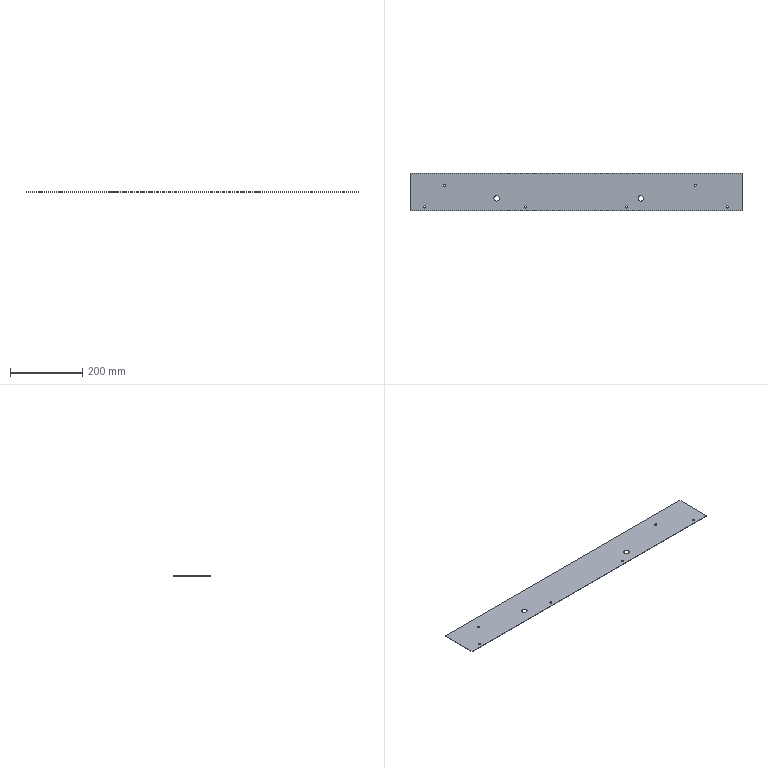Part | SolidWorks | features Cut 1, Extrusion 1, HoleWzd 1 | 1 solid | 22 faces | box 920 x 105 x 1 mm | volume 96077 mm3 | cylinder 16 | plane 6 | commonest cylinder face diameters 6 x12 15 x4
STEP:
#1=CARTESIAN_POINT('',(-423.,-41.5,-0.5));
#2=VERTEX_POINT('',#1);
#3=CARTESIAN_POINT('',(-417.,-41.5,-0.5));
#4=VERTEX_POINT('',#3);
#5=CARTESIAN_POINT('',(-420.,-41.5,-0.5));
#6=DIRECTION('',(0.,0.,1.));
#7=DIRECTION('',(1.,0.,0.));
#8=AXIS2_PLACEMENT_3D('',#5,#6,#7);
#9=CIRCLE('',#8,3.);
#10=EDGE_CURVE('',#2,#4,#9,.T.);
#11=ORIENTED_EDGE('',*,*,#10,.F.);
#12=CARTESIAN_POINT('',(-423.,-41.5,0.5));
#13=VERTEX_POINT('',#12);
#14=CARTESIAN_POINT('',(-423.,-41.5,0.5));
#15=DIRECTION('',(0.,0.,1.));
#16=VECTOR('',#15,1000.);
#17=LINE('',#14,#16);
#18=EDGE_CURVE('',#2,#13,#17,.T.);
#19=ORIENTED_EDGE('',*,*,#18,.T.);
#20=CARTESIAN_POINT('',(-417.,-41.5,0.5));
#21=VERTEX_POINT('',#20);
#22=CARTESIAN_POINT('',(-420.,-41.5,0.5));
#23=DIRECTION('',(0.,0.,1.));
#24=DIRECTION('',(1.,0.,0.));
#25=AXIS2_PLACEMENT_3D('',#22,#23,#24);
#26=CIRCLE('',#25,3.);
#27=EDGE_CURVE('',#13,#21,#26,.T.);
#28=ORIENTED_EDGE('',*,*,#27,.T.);
#29=CARTESIAN_POINT('',(-417.,-41.5,0.5));
#30=DIRECTION('',(0.,0.,1.));
#31=VECTOR('',#30,1000.);
#32=LINE('',#29,#31);
#33=EDGE_CURVE('',#4,#21,#32,.T.);
#34=ORIENTED_EDGE('',*,*,#33,.F.);
#35=EDGE_LOOP('',(#11,#19,#28,#34));
#36=FACE_OUTER_BOUND('',#35,.T.);
#37=CARTESIAN_POINT('',(-420.,-41.5,0.5));
#38=DIRECTION('',(0.,0.,1.));
#39=DIRECTION('',(1.,0.,0.));
#40=AXIS2_PLACEMENT_3D('',#37,#38,#39);
#41=CYLINDRICAL_SURFACE('',#40,3.);
#42=ADVANCED_FACE('',(#36),#41,.F.);
#43=CARTESIAN_POINT('',(-143.,-41.5,-0.5));
#44=VERTEX_POINT('',#43);
#45=CARTESIAN_POINT('',(-137.,-41.5,-0.5));
#46=VERTEX_POINT('',#45);
#47=CARTESIAN_POINT('',(-140.,-41.5,-0.5));
#48=DIRECTION('',(0.,0.,1.));
#49=DIRECTION('',(1.,0.,0.));
#50=AXIS2_PLACEMENT_3D('',#47,#48,#49);
#51=CIRCLE('',#50,3.);
#52=EDGE_CURVE('',#44,#46,#51,.T.);
#53=ORIENTED_EDGE('',*,*,#52,.F.);
#54=CARTESIAN_POINT('',(-143.,-41.5,0.5));
#55=VERTEX_POINT('',#54);
#56=CARTESIAN_POINT('',(-143.,-41.5,0.5));
#57=DIRECTION('',(0.,0.,1.));
#58=VECTOR('',#57,1000.);
#59=LINE('',#56,#58);
#60=EDGE_CURVE('',#44,#55,#59,.T.);
#61=ORIENTED_EDGE('',*,*,#60,.T.);
#62=CARTESIAN_POINT('',(-137.,-41.5,0.5));
#63=VERTEX_POINT('',#62);
#64=CARTESIAN_POINT('',(-140.,-41.5,0.5));
#65=DIRECTION('',(0.,0.,1.));
#66=DIRECTION('',(1.,0.,0.));
#67=AXIS2_PLACEMENT_3D('',#64,#65,#66);
#68=CIRCLE('',#67,3.);
#69=EDGE_CURVE('',#55,#63,#68,.T.);
#70=ORIENTED_EDGE('',*,*,#69,.T.);
#71=CARTESIAN_POINT('',(-137.,-41.5,0.5));
#72=DIRECTION('',(0.,0.,1.));
#73=VECTOR('',#72,1000.);
#74=LINE('',#71,#73);
#75=EDGE_CURVE('',#46,#63,#74,.T.);
#76=ORIENTED_EDGE('',*,*,#75,.F.);
#77=EDGE_LOOP('',(#53,#61,#70,#76));
#78=FACE_OUTER_BOUND('',#77,.T.);
#79=CARTESIAN_POINT('',(-140.,-41.5,0.5));
#80=DIRECTION('',(0.,0.,1.));
#81=DIRECTION('',(1.,0.,0.));
#82=AXIS2_PLACEMENT_3D('',#79,#80,#81);
#83=CYLINDRICAL_SURFACE('',#82,3.);
#84=ADVANCED_FACE('',(#78),#83,.F.);
#85=CARTESIAN_POINT('',(137.,-41.5,-0.5));
#86=VERTEX_POINT('',#85);
#87=CARTESIAN_POINT('',(143.,-41.5,-0.5));
#88=VERTEX_POINT('',#87);
#89=CARTESIAN_POINT('',(140.,-41.5,-0.5));
#90=DIRECTION('',(0.,0.,1.));
#91=DIRECTION('',(1.,0.,0.));
#92=AXIS2_PLACEMENT_3D('',#89,#90,#91);
#93=CIRCLE('',#92,3.);
#94=EDGE_CURVE('',#86,#88,#93,.T.);
#95=ORIENTED_EDGE('',*,*,#94,.F.);
#96=CARTESIAN_POINT('',(137.,-41.5,0.5));
#97=VERTEX_POINT('',#96);
#98=CARTESIAN_POINT('',(137.,-41.5,0.5));
#99=DIRECTION('',(0.,0.,1.));
#100=VECTOR('',#99,1000.);
#101=LINE('',#98,#100);
#102=EDGE_CURVE('',#86,#97,#101,.T.);
#103=ORIENTED_EDGE('',*,*,#102,.T.);
#104=CARTESIAN_POINT('',(143.,-41.5,0.5));
#105=VERTEX_POINT('',#104);
#106=CARTESIAN_POINT('',(140.,-41.5,0.5));
#107=DIRECTION('',(0.,0.,1.));
#108=DIRECTION('',(1.,0.,0.));
#109=AXIS2_PLACEMENT_3D('',#106,#107,#108);
#110=CIRCLE('',#109,3.);
#111=EDGE_CURVE('',#97,#105,#110,.T.);
#112=ORIENTED_EDGE('',*,*,#111,.T.);
#113=CARTESIAN_POINT('',(143.,-41.5,0.5));
#114=DIRECTION('',(0.,0.,1.));
#115=VECTOR('',#114,1000.);
#116=LINE('',#113,#115);
#117=EDGE_CURVE('',#88,#105,#116,.T.);
#118=ORIENTED_EDGE('',*,*,#117,.F.);
#119=EDGE_LOOP('',(#95,#103,#112,#118));
#120=FACE_OUTER_BOUND('',#119,.T.);
#121=CARTESIAN_POINT('',(140.,-41.5,0.5));
#122=DIRECTION('',(0.,0.,1.));
#123=DIRECTION('',(1.,0.,0.));
#124=AXIS2_PLACEMENT_3D('',#121,#122,#123);
#125=CYLINDRICAL_SURFACE('',#124,3.);
#126=ADVANCED_FACE('',(#120),#125,.F.);
#127=CARTESIAN_POINT('',(-368.,18.5,-0.5));
#128=VERTEX_POINT('',#127);
#129=CARTESIAN_POINT('',(-362.,18.5,-0.5));
#130=VERTEX_POINT('',#129);
#131=CARTESIAN_POINT('',(-365.,18.5,-0.5));
#132=DIRECTION('',(0.,0.,1.));
#133=DIRECTION('',(1.,0.,0.));
#134=AXIS2_PLACEMENT_3D('',#131,#132,#133);
#135=CIRCLE('',#134,3.);
#136=EDGE_CURVE('',#128,#130,#135,.T.);
#137=ORIENTED_EDGE('',*,*,#136,.F.);
#138=CARTESIAN_POINT('',(-368.,18.5,0.5));
#139=VERTEX_POINT('',#138);
#140=CARTESIAN_POINT('',(-368.,18.5,0.5));
#141=DIRECTION('',(0.,0.,1.));
#142=VECTOR('',#141,1000.);
#143=LINE('',#140,#142);
#144=EDGE_CURVE('',#128,#139,#143,.T.);
#145=ORIENTED_EDGE('',*,*,#144,.T.);
#146=CARTESIAN_POINT('',(-362.,18.5,0.5));
#147=VERTEX_POINT('',#146);
#148=CARTESIAN_POINT('',(-365.,18.5,0.5));
#149=DIRECTION('',(0.,0.,1.));
#150=DIRECTION('',(1.,0.,0.));
#151=AXIS2_PLACEMENT_3D('',#148,#149,#150);
#152=CIRCLE('',#151,3.);
#153=EDGE_CURVE('',#139,#147,#152,.T.);
#154=ORIENTED_EDGE('',*,*,#153,.T.);
#155=CARTESIAN_POINT('',(-362.,18.5,0.5));
#156=DIRECTION('',(0.,0.,1.));
#157=VECTOR('',#156,1000.);
#158=LINE('',#155,#157);
#159=EDGE_CURVE('',#130,#147,#158,.T.);
#160=ORIENTED_EDGE('',*,*,#159,.F.);
#161=EDGE_LOOP('',(#137,#145,#154,#160));
#162=FACE_OUTER_BOUND('',#161,.T.);
#163=CARTESIAN_POINT('',(-365.,18.5,0.5));
#164=DIRECTION('',(0.,0.,1.));
#165=DIRECTION('',(1.,0.,0.));
#166=AXIS2_PLACEMENT_3D('',#163,#164,#165);
#167=CYLINDRICAL_SURFACE('',#166,3.);
#168=ADVANCED_FACE('',(#162),#167,.F.);
#169=CARTESIAN_POINT('',(327.,18.5,-0.5));
#170=VERTEX_POINT('',#169);
#171=CARTESIAN_POINT('',(333.,18.5,-0.5));
#172=VERTEX_POINT('',#171);
#173=CARTESIAN_POINT('',(330.,18.5,-0.5));
#174=DIRECTION('',(0.,0.,1.));
#175=DIRECTION('',(1.,0.,0.));
#176=AXIS2_PLACEMENT_3D('',#173,#174,#175);
#177=CIRCLE('',#176,3.);
#178=EDGE_CURVE('',#170,#172,#177,.T.);
#179=ORIENTED_EDGE('',*,*,#178,.F.);
#180=CARTESIAN_POINT('',(327.,18.5,0.5));
#181=VERTEX_POINT('',#180);
#182=CARTESIAN_POINT('',(327.,18.5,0.5));
#183=DIRECTION('',(0.,0.,1.));
#184=VECTOR('',#183,1000.);
#185=LINE('',#182,#184);
#186=EDGE_CURVE('',#170,#181,#185,.T.);
#187=ORIENTED_EDGE('',*,*,#186,.T.);
#188=CARTESIAN_POINT('',(333.,18.5,0.5));
#189=VERTEX_POINT('',#188);
#190=CARTESIAN_POINT('',(330.,18.5,0.5));
#191=DIRECTION('',(0.,0.,1.));
#192=DIRECTION('',(1.,0.,0.));
#193=AXIS2_PLACEMENT_3D('',#190,#191,#192);
#194=CIRCLE('',#193,3.);
#195=EDGE_CURVE('',#181,#189,#194,.T.);
#196=ORIENTED_EDGE('',*,*,#195,.T.);
#197=CARTESIAN_POINT('',(333.,18.5,0.5));
#198=DIRECTION('',(0.,0.,1.));
#199=VECTOR('',#198,1000.);
#200=LINE('',#197,#199);
#201=EDGE_CURVE('',#172,#189,#200,.T.);
#202=ORIENTED_EDGE('',*,*,#201,.F.);
#203=EDGE_LOOP('',(#179,#187,#196,#202));
#204=FACE_OUTER_BOUND('',#203,.T.);
#205=CARTESIAN_POINT('',(330.,18.5,0.5));
#206=DIRECTION('',(0.,0.,1.));
#207=DIRECTION('',(1.,0.,0.));
#208=AXIS2_PLACEMENT_3D('',#205,#206,#207);
#209=CYLINDRICAL_SURFACE('',#208,3.);
#210=ADVANCED_FACE('',(#204),#209,.F.);
#211=CARTESIAN_POINT('',(417.,-41.5,-0.5));
#212=VERTEX_POINT('',#211);
#213=CARTESIAN_POINT('',(423.,-41.5,-0.5));
#214=VERTEX_POINT('',#213);
#215=CARTESIAN_POINT('',(420.,-41.5,-0.5));
#216=DIRECTION('',(0.,0.,1.));
#217=DIRECTION('',(1.,0.,0.));
#218=AXIS2_PLACEMENT_3D('',#215,#216,#217);
#219=CIRCLE('',#218,3.);
#220=EDGE_CURVE('',#212,#214,#219,.T.);
#221=ORIENTED_EDGE('',*,*,#220,.F.);
#222=CARTESIAN_POINT('',(417.,-41.5,0.5));
#223=VERTEX_POINT('',#222);
#224=CARTESIAN_POINT('',(417.,-41.5,0.5));
#225=DIRECTION('',(0.,0.,1.));
#226=VECTOR('',#225,1000.);
#227=LINE('',#224,#226);
#228=EDGE_CURVE('',#212,#223,#227,.T.);
#229=ORIENTED_EDGE('',*,*,#228,.T.);
#230=CARTESIAN_POINT('',(423.,-41.5,0.5));
#231=VERTEX_POINT('',#230);
#232=CARTESIAN_POINT('',(420.,-41.5,0.5));
#233=DIRECTION('',(0.,0.,1.));
#234=DIRECTION('',(1.,0.,0.));
#235=AXIS2_PLACEMENT_3D('',#232,#233,#234);
#236=CIRCLE('',#235,3.);
#237=EDGE_CURVE('',#223,#231,#236,.T.);
#238=ORIENTED_EDGE('',*,*,#237,.T.);
#239=CARTESIAN_POINT('',(423.,-41.5,0.5));
#240=DIRECTION('',(0.,0.,1.));
#241=VECTOR('',#240,1000.);
#242=LINE('',#239,#241);
#243=EDGE_CURVE('',#214,#231,#242,.T.);
#244=ORIENTED_EDGE('',*,*,#243,.F.);
#245=EDGE_LOOP('',(#221,#229,#238,#244));
#246=FACE_OUTER_BOUND('',#245,.T.);
#247=CARTESIAN_POINT('',(420.,-41.5,0.5));
#248=DIRECTION('',(0.,0.,1.));
#249=DIRECTION('',(1.,0.,0.));
#250=AXIS2_PLACEMENT_3D('',#247,#248,#249);
#251=CYLINDRICAL_SURFACE('',#250,3.);
#252=ADVANCED_FACE('',(#246),#251,.F.);
#253=CARTESIAN_POINT('',(172.5,-17.5,-0.5));
#254=VERTEX_POINT('',#253);
#255=CARTESIAN_POINT('',(187.5,-17.5,-0.5));
#256=VERTEX_POINT('',#255);
#257=CARTESIAN_POINT('',(180.,-17.5,-0.5));
#258=DIRECTION('',(0.,0.,1.));
#259=DIRECTION('',(1.,0.,0.));
#260=AXIS2_PLACEMENT_3D('',#257,#258,#259);
#261=CIRCLE('',#260,7.5);
#262=EDGE_CURVE('',#254,#256,#261,.T.);
#263=ORIENTED_EDGE('',*,*,#262,.F.);
#264=CARTESIAN_POINT('',(172.5,-17.5,0.5));
#265=VERTEX_POINT('',#264);
#266=CARTESIAN_POINT('',(172.5,-17.5,-0.5));
#267=DIRECTION('',(0.,0.,1.));
#268=VECTOR('',#267,1000.);
#269=LINE('',#266,#268);
#270=EDGE_CURVE('',#254,#265,#269,.T.);
#271=ORIENTED_EDGE('',*,*,#270,.T.);
#272=CARTESIAN_POINT('',(187.5,-17.5,0.5));
#273=VERTEX_POINT('',#272);
#274=CARTESIAN_POINT('',(180.,-17.5,0.5));
#275=DIRECTION('',(0.,0.,1.));
#276=DIRECTION('',(1.,0.,0.));
#277=AXIS2_PLACEMENT_3D('',#274,#275,#276);
#278=CIRCLE('',#277,7.5);
#279=EDGE_CURVE('',#265,#273,#278,.T.);
#280=ORIENTED_EDGE('',*,*,#279,.T.);
#281=CARTESIAN_POINT('',(187.5,-17.5,-0.5));
#282=DIRECTION('',(0.,0.,1.));
#283=VECTOR('',#282,1000.);
#284=LINE('',#281,#283);
#285=EDGE_CURVE('',#256,#273,#284,.T.);
#286=ORIENTED_EDGE('',*,*,#285,.F.);
#287=EDGE_LOOP('',(#263,#271,#280,#286));
#288=FACE_OUTER_BOUND('',#287,.T.);
#289=CARTESIAN_POINT('',(180.,-17.5,-0.5));
#290=DIRECTION('',(0.,0.,1.));
#291=DIRECTION('',(1.,0.,0.));
#292=AXIS2_PLACEMENT_3D('',#289,#290,#291);
#293=CYLINDRICAL_SURFACE('',#292,7.5);
#294=ADVANCED_FACE('',(#288),#293,.F.);
#295=CARTESIAN_POINT('',(-227.5,-17.5,-0.5));
#296=VERTEX_POINT('',#295);
#297=CARTESIAN_POINT('',(-212.5,-17.5,-0.5));
#298=VERTEX_POINT('',#297);
#299=CARTESIAN_POINT('',(-220.,-17.5,-0.5));
#300=DIRECTION('',(0.,0.,1.));
#301=DIRECTION('',(1.,0.,0.));
#302=AXIS2_PLACEMENT_3D('',#299,#300,#301);
#303=CIRCLE('',#302,7.5);
#304=EDGE_CURVE('',#296,#298,#303,.T.);
#305=ORIENTED_EDGE('',*,*,#304,.F.);
#306=CARTESIAN_POINT('',(-227.5,-17.5,0.5));
#307=VERTEX_POINT('',#306);
#308=CARTESIAN_POINT('',(-227.5,-17.5,-0.5));
#309=DIRECTION('',(0.,0.,1.));
#310=VECTOR('',#309,1000.);
#311=LINE('',#308,#310);
#312=EDGE_CURVE('',#296,#307,#311,.T.);
#313=ORIENTED_EDGE('',*,*,#312,.T.);
#314=CARTESIAN_POINT('',(-212.5,-17.5,0.5));
#315=VERTEX_POINT('',#314);
#316=CARTESIAN_POINT('',(-220.,-17.5,0.5));
#317=DIRECTION('',(0.,0.,1.));
#318=DIRECTION('',(1.,0.,0.));
#319=AXIS2_PLACEMENT_3D('',#316,#317,#318);
#320=CIRCLE('',#319,7.5);
#321=EDGE_CURVE('',#307,#315,#320,.T.);
#322=ORIENTED_EDGE('',*,*,#321,.T.);
#323=CARTESIAN_POINT('',(-212.5,-17.5,-0.5));
#324=DIRECTION('',(0.,0.,1.));
#325=VECTOR('',#324,1000.);
#326=LINE('',#323,#325);
#327=EDGE_CURVE('',#298,#315,#326,.T.);
#328=ORIENTED_EDGE('',*,*,#327,.F.);
#329=EDGE_LOOP('',(#305,#313,#322,#328));
#330=FACE_OUTER_BOUND('',#329,.T.);
#331=CARTESIAN_POINT('',(-220.,-17.5,-0.5));
#332=DIRECTION('',(0.,0.,1.));
#333=DIRECTION('',(1.,0.,0.));
#334=AXIS2_PLACEMENT_3D('',#331,#332,#333);
#335=CYLINDRICAL_SURFACE('',#334,7.5);
#336=ADVANCED_FACE('',(#330),#335,.F.);
#337=CARTESIAN_POINT('',(-460.,-52.5,-0.5));
#338=VERTEX_POINT('',#337);
#339=CARTESIAN_POINT('',(-460.,-52.5,0.5));
#340=VERTEX_POINT('',#339);
#341=CARTESIAN_POINT('',(-460.,-52.5,-0.5));
#342=DIRECTION('',(0.,0.,1.));
#343=VECTOR('',#342,1000.);
#344=LINE('',#341,#343);
#345=EDGE_CURVE('',#338,#340,#344,.T.);
#346=ORIENTED_EDGE('',*,*,#345,.T.);
#347=CARTESIAN_POINT('',(-460.,52.5,0.5));
#348=VERTEX_POINT('',#347);
#349=CARTESIAN_POINT('',(-460.,52.5,0.5));
#350=DIRECTION('',(0.,-1.,0.));
#351=VECTOR('',#350,1000.);
#352=LINE('',#349,#351);
#353=EDGE_CURVE('',#348,#340,#352,.T.);
#354=ORIENTED_EDGE('',*,*,#353,.F.);
#355=CARTESIAN_POINT('',(-460.,52.5,-0.5));
#356=VERTEX_POINT('',#355);
#357=CARTESIAN_POINT('',(-460.,52.5,-0.5));
#358=DIRECTION('',(0.,0.,1.));
#359=VECTOR('',#358,1000.);
#360=LINE('',#357,#359);
#361=EDGE_CURVE('',#356,#348,#360,.T.);
#362=ORIENTED_EDGE('',*,*,#361,.F.);
#363=CARTESIAN_POINT('',(-460.,52.5,-0.5));
#364=DIRECTION('',(0.,-1.,0.));
#365=VECTOR('',#364,1000.);
#366=LINE('',#363,#365);
#367=EDGE_CURVE('',#356,#338,#366,.T.);
#368=ORIENTED_EDGE('',*,*,#367,.T.);
#369=EDGE_LOOP('',(#346,#354,#362,#368));
#370=FACE_OUTER_BOUND('',#369,.T.);
#371=CARTESIAN_POINT('',(-460.,52.5,-0.5));
#372=DIRECTION('',(1.,0.,0.));
#373=DIRECTION('',(0.,0.,-1.));
#374=AXIS2_PLACEMENT_3D('',#371,#372,#373);
#375=PLANE('',#374);
#376=ADVANCED_FACE('',(#370),#375,.F.);
#377=CARTESIAN_POINT('',(-420.,-41.5,0.5));
#378=DIRECTION('',(0.,0.,1.));
#379=DIRECTION('',(1.,0.,0.));
#380=AXIS2_PLACEMENT_3D('',#377,#378,#379);
#381=CIRCLE('',#380,3.);
#382=EDGE_CURVE('',#21,#13,#381,.T.);
#383=ORIENTED_EDGE('',*,*,#382,.F.);
#384=ORIENTED_EDGE('',*,*,#27,.F.);
#385=EDGE_LOOP('',(#383,#384));
#386=FACE_BOUND('',#385,.T.);
#387=CARTESIAN_POINT('',(-140.,-41.5,0.5));
#388=DIRECTION('',(0.,0.,1.));
#389=DIRECTION('',(1.,0.,0.));
#390=AXIS2_PLACEMENT_3D('',#387,#388,#389);
#391=CIRCLE('',#390,3.);
#392=EDGE_CURVE('',#63,#55,#391,.T.);
#393=ORIENTED_EDGE('',*,*,#392,.F.);
#394=ORIENTED_EDGE('',*,*,#69,.F.);
#395=EDGE_LOOP('',(#393,#394));
#396=FACE_BOUND('',#395,.T.);
#397=CARTESIAN_POINT('',(140.,-41.5,0.5));
#398=DIRECTION('',(0.,0.,1.));
#399=DIRECTION('',(1.,0.,0.));
#400=AXIS2_PLACEMENT_3D('',#397,#398,#399);
#401=CIRCLE('',#400,3.);
#402=EDGE_CURVE('',#105,#97,#401,.T.);
#403=ORIENTED_EDGE('',*,*,#402,.F.);
#404=ORIENTED_EDGE('',*,*,#111,.F.);
#405=EDGE_LOOP('',(#403,#404));
#406=FACE_BOUND('',#405,.T.);
#407=CARTESIAN_POINT('',(-365.,18.5,0.5));
#408=DIRECTION('',(0.,0.,1.));
#409=DIRECTION('',(1.,0.,0.));
#410=AXIS2_PLACEMENT_3D('',#407,#408,#409);
#411=CIRCLE('',#410,3.);
#412=EDGE_CURVE('',#147,#139,#411,.T.);
#413=ORIENTED_EDGE('',*,*,#412,.F.);
#414=ORIENTED_EDGE('',*,*,#153,.F.);
#415=EDGE_LOOP('',(#413,#414));
#416=FACE_BOUND('',#415,.T.);
#417=CARTESIAN_POINT('',(330.,18.5,0.5));
#418=DIRECTION('',(0.,0.,1.));
#419=DIRECTION('',(1.,0.,0.));
#420=AXIS2_PLACEMENT_3D('',#417,#418,#419);
#421=CIRCLE('',#420,3.);
#422=EDGE_CURVE('',#189,#181,#421,.T.);
#423=ORIENTED_EDGE('',*,*,#422,.F.);
#424=ORIENTED_EDGE('',*,*,#195,.F.);
#425=EDGE_LOOP('',(#423,#424));
#426=FACE_BOUND('',#425,.T.);
#427=CARTESIAN_POINT('',(420.,-41.5,0.5));
#428=DIRECTION('',(0.,0.,1.));
#429=DIRECTION('',(1.,0.,0.));
#430=AXIS2_PLACEMENT_3D('',#427,#428,#429);
#431=CIRCLE('',#430,3.);
#432=EDGE_CURVE('',#231,#223,#431,.T.);
#433=ORIENTED_EDGE('',*,*,#432,.F.);
#434=ORIENTED_EDGE('',*,*,#237,.F.);
#435=EDGE_LOOP('',(#433,#434));
#436=FACE_BOUND('',#435,.T.);
#437=CARTESIAN_POINT('',(180.,-17.5,0.5));
#438=DIRECTION('',(0.,0.,1.));
#439=DIRECTION('',(1.,0.,0.));
#440=AXIS2_PLACEMENT_3D('',#437,#438,#439);
#441=CIRCLE('',#440,7.5);
#442=EDGE_CURVE('',#273,#265,#441,.T.);
#443=ORIENTED_EDGE('',*,*,#442,.F.);
#444=ORIENTED_EDGE('',*,*,#279,.F.);
#445=EDGE_LOOP('',(#443,#444));
#446=FACE_BOUND('',#445,.T.);
#447=CARTESIAN_POINT('',(-220.,-17.5,0.5));
#448=DIRECTION('',(0.,0.,1.));
#449=DIRECTION('',(1.,0.,0.));
#450=AXIS2_PLACEMENT_3D('',#447,#448,#449);
#451=CIRCLE('',#450,7.5);
#452=EDGE_CURVE('',#315,#307,#451,.T.);
#453=ORIENTED_EDGE('',*,*,#452,.F.);
#454=ORIENTED_EDGE('',*,*,#321,.F.);
#455=EDGE_LOOP('',(#453,#454));
#456=FACE_BOUND('',#455,.T.);
#457=CARTESIAN_POINT('',(460.,-52.5,0.5));
#458=VERTEX_POINT('',#457);
#459=CARTESIAN_POINT('',(-460.,-52.5,0.5));
#460=DIRECTION('',(1.,0.,0.));
#461=VECTOR('',#460,1000.);
#462=LINE('',#459,#461);
#463=EDGE_CURVE('',#340,#458,#462,.T.);
#464=ORIENTED_EDGE('',*,*,#463,.T.);
#465=CARTESIAN_POINT('',(460.,52.5,0.5));
#466=VERTEX_POINT('',#465);
#467=CARTESIAN_POINT('',(460.,52.5,0.5));
#468=DIRECTION('',(0.,-1.,0.));
#469=VECTOR('',#468,1000.);
#470=LINE('',#467,#469);
#471=EDGE_CURVE('',#466,#458,#470,.T.);
#472=ORIENTED_EDGE('',*,*,#471,.F.);
#473=CARTESIAN_POINT('',(-460.,52.5,0.5));
#474=DIRECTION('',(1.,0.,0.));
#475=VECTOR('',#474,1000.);
#476=LINE('',#473,#475);
#477=EDGE_CURVE('',#348,#466,#476,.T.);
#478=ORIENTED_EDGE('',*,*,#477,.F.);
#479=ORIENTED_EDGE('',*,*,#353,.T.);
#480=EDGE_LOOP('',(#464,#472,#478,#479));
#481=FACE_OUTER_BOUND('',#480,.T.);
#482=CARTESIAN_POINT('',(-460.,52.5,0.5));
#483=DIRECTION('',(0.,0.,-1.));
#484=DIRECTION('',(-1.,0.,0.));
#485=AXIS2_PLACEMENT_3D('',#482,#483,#484);
#486=PLANE('',#485);
#487=ADVANCED_FACE('',(#386,#396,#406,#416,#426,#436,#446,#456,#481),#486,.F.);
#488=CARTESIAN_POINT('',(460.,-52.5,-0.5));
#489=VERTEX_POINT('',#488);
#490=CARTESIAN_POINT('',(460.,-52.5,-0.5));
#491=DIRECTION('',(0.,0.,-1.));
#492=VECTOR('',#491,1000.);
#493=LINE('',#490,#492);
#494=EDGE_CURVE('',#458,#489,#493,.T.);
#495=ORIENTED_EDGE('',*,*,#494,.T.);
#496=CARTESIAN_POINT('',(460.,52.5,-0.5));
#497=VERTEX_POINT('',#496);
#498=CARTESIAN_POINT('',(460.,52.5,-0.5));
#499=DIRECTION('',(0.,-1.,0.));
#500=VECTOR('',#499,1000.);
#501=LINE('',#498,#500);
#502=EDGE_CURVE('',#497,#489,#501,.T.);
#503=ORIENTED_EDGE('',*,*,#502,.F.);
#504=CARTESIAN_POINT('',(460.,52.5,-0.5));
#505=DIRECTION('',(0.,0.,-1.));
#506=VECTOR('',#505,1000.);
#507=LINE('',#504,#506);
#508=EDGE_CURVE('',#466,#497,#507,.T.);
#509=ORIENTED_EDGE('',*,*,#508,.F.);
#510=ORIENTED_EDGE('',*,*,#471,.T.);
#511=EDGE_LOOP('',(#495,#503,#509,#510));
#512=FACE_OUTER_BOUND('',#511,.T.);
#513=CARTESIAN_POINT('',(460.,52.5,-0.5));
#514=DIRECTION('',(-1.,0.,0.));
#515=DIRECTION('',(0.,0.,1.));
#516=AXIS2_PLACEMENT_3D('',#513,#514,#515);
#517=PLANE('',#516);
#518=ADVANCED_FACE('',(#512),#517,.F.);
#519=CARTESIAN_POINT('',(-420.,-41.5,-0.5));
#520=DIRECTION('',(0.,0.,1.));
#521=DIRECTION('',(1.,0.,0.));
#522=AXIS2_PLACEMENT_3D('',#519,#520,#521);
#523=CIRCLE('',#522,3.);
#524=EDGE_CURVE('',#4,#2,#523,.T.);
#525=ORIENTED_EDGE('',*,*,#524,.T.);
#526=ORIENTED_EDGE('',*,*,#10,.T.);
#527=EDGE_LOOP('',(#525,#526));
#528=FACE_BOUND('',#527,.T.);
#529=CARTESIAN_POINT('',(-140.,-41.5,-0.5));
#530=DIRECTION('',(0.,0.,1.));
#531=DIRECTION('',(1.,0.,0.));
#532=AXIS2_PLACEMENT_3D('',#529,#530,#531);
#533=CIRCLE('',#532,3.);
#534=EDGE_CURVE('',#46,#44,#533,.T.);
#535=ORIENTED_EDGE('',*,*,#534,.T.);
#536=ORIENTED_EDGE('',*,*,#52,.T.);
#537=EDGE_LOOP('',(#535,#536));
#538=FACE_BOUND('',#537,.T.);
#539=CARTESIAN_POINT('',(140.,-41.5,-0.5));
#540=DIRECTION('',(0.,0.,1.));
#541=DIRECTION('',(1.,0.,0.));
#542=AXIS2_PLACEMENT_3D('',#539,#540,#541);
#543=CIRCLE('',#542,3.);
#544=EDGE_CURVE('',#88,#86,#543,.T.);
#545=ORIENTED_EDGE('',*,*,#544,.T.);
#546=ORIENTED_EDGE('',*,*,#94,.T.);
#547=EDGE_LOOP('',(#545,#546));
#548=FACE_BOUND('',#547,.T.);
#549=CARTESIAN_POINT('',(-365.,18.5,-0.5));
#550=DIRECTION('',(0.,0.,1.));
#551=DIRECTION('',(1.,0.,0.));
#552=AXIS2_PLACEMENT_3D('',#549,#550,#551);
#553=CIRCLE('',#552,3.);
#554=EDGE_CURVE('',#130,#128,#553,.T.);
#555=ORIENTED_EDGE('',*,*,#554,.T.);
#556=ORIENTED_EDGE('',*,*,#136,.T.);
#557=EDGE_LOOP('',(#555,#556));
#558=FACE_BOUND('',#557,.T.);
#559=CARTESIAN_POINT('',(330.,18.5,-0.5));
#560=DIRECTION('',(0.,0.,1.));
#561=DIRECTION('',(1.,0.,0.));
#562=AXIS2_PLACEMENT_3D('',#559,#560,#561);
#563=CIRCLE('',#562,3.);
#564=EDGE_CURVE('',#172,#170,#563,.T.);
#565=ORIENTED_EDGE('',*,*,#564,.T.);
#566=ORIENTED_EDGE('',*,*,#178,.T.);
#567=EDGE_LOOP('',(#565,#566));
#568=FACE_BOUND('',#567,.T.);
#569=CARTESIAN_POINT('',(420.,-41.5,-0.5));
#570=DIRECTION('',(0.,0.,1.));
#571=DIRECTION('',(1.,0.,0.));
#572=AXIS2_PLACEMENT_3D('',#569,#570,#571);
#573=CIRCLE('',#572,3.);
#574=EDGE_CURVE('',#214,#212,#573,.T.);
#575=ORIENTED_EDGE('',*,*,#574,.T.);
#576=ORIENTED_EDGE('',*,*,#220,.T.);
#577=EDGE_LOOP('',(#575,#576));
#578=FACE_BOUND('',#577,.T.);
#579=CARTESIAN_POINT('',(180.,-17.5,-0.5));
#580=DIRECTION('',(0.,0.,1.));
#581=DIRECTION('',(1.,0.,0.));
#582=AXIS2_PLACEMENT_3D('',#579,#580,#581);
#583=CIRCLE('',#582,7.5);
#584=EDGE_CURVE('',#256,#254,#583,.T.);
#585=ORIENTED_EDGE('',*,*,#584,.T.);
#586=ORIENTED_EDGE('',*,*,#262,.T.);
#587=EDGE_LOOP('',(#585,#586));
#588=FACE_BOUND('',#587,.T.);
#589=CARTESIAN_POINT('',(-220.,-17.5,-0.5));
#590=DIRECTION('',(0.,0.,1.));
#591=DIRECTION('',(1.,0.,0.));
#592=AXIS2_PLACEMENT_3D('',#589,#590,#591);
#593=CIRCLE('',#592,7.5);
#594=EDGE_CURVE('',#298,#296,#593,.T.);
#595=ORIENTED_EDGE('',*,*,#594,.T.);
#596=ORIENTED_EDGE('',*,*,#304,.T.);
#597=EDGE_LOOP('',(#595,#596));
#598=FACE_BOUND('',#597,.T.);
#599=CARTESIAN_POINT('',(-460.,-52.5,-0.5));
#600=DIRECTION('',(-1.,0.,0.));
#601=VECTOR('',#600,1000.);
#602=LINE('',#599,#601);
#603=EDGE_CURVE('',#489,#338,#602,.T.);
#604=ORIENTED_EDGE('',*,*,#603,.T.);
#605=ORIENTED_EDGE('',*,*,#367,.F.);
#606=CARTESIAN_POINT('',(-460.,52.5,-0.5));
#607=DIRECTION('',(-1.,0.,0.));
#608=VECTOR('',#607,1000.);
#609=LINE('',#606,#608);
#610=EDGE_CURVE('',#497,#356,#609,.T.);
#611=ORIENTED_EDGE('',*,*,#610,.F.);
#612=ORIENTED_EDGE('',*,*,#502,.T.);
#613=EDGE_LOOP('',(#604,#605,#611,#612));
#614=FACE_OUTER_BOUND('',#613,.T.);
#615=CARTESIAN_POINT('',(-460.,52.5,-0.5));
#616=DIRECTION('',(0.,0.,1.));
#617=DIRECTION('',(1.,0.,0.));
#618=AXIS2_PLACEMENT_3D('',#615,#616,#617);
#619=PLANE('',#618);
#620=ADVANCED_FACE('',(#528,#538,#548,#558,#568,#578,#588,#598,#614),#619,.F.);
#621=ORIENTED_EDGE('',*,*,#361,.T.);
#622=ORIENTED_EDGE('',*,*,#477,.T.);
#623=ORIENTED_EDGE('',*,*,#508,.T.);
#624=ORIENTED_EDGE('',*,*,#610,.T.);
#625=EDGE_LOOP('',(#621,#622,#623,#624));
#626=FACE_OUTER_BOUND('',#625,.T.);
#627=CARTESIAN_POINT('',(-460.,52.5,0.5));
#628=DIRECTION('',(0.,1.,0.));
#629=DIRECTION('',(0.,0.,1.));
#630=AXIS2_PLACEMENT_3D('',#627,#628,#629);
#631=PLANE('',#630);
#632=ADVANCED_FACE('',(#626),#631,.T.);
#633=ORIENTED_EDGE('',*,*,#345,.F.);
#634=ORIENTED_EDGE('',*,*,#603,.F.);
#635=ORIENTED_EDGE('',*,*,#494,.F.);
#636=ORIENTED_EDGE('',*,*,#463,.F.);
#637=EDGE_LOOP('',(#633,#634,#635,#636));
#638=FACE_OUTER_BOUND('',#637,.T.);
#639=CARTESIAN_POINT('',(-460.,-52.5,0.5));
#640=DIRECTION('',(0.,1.,0.));
#641=DIRECTION('',(0.,0.,1.));
#642=AXIS2_PLACEMENT_3D('',#639,#640,#641);
#643=PLANE('',#642);
#644=ADVANCED_FACE('',(#638),#643,.F.);
#645=ORIENTED_EDGE('',*,*,#312,.F.);
#646=ORIENTED_EDGE('',*,*,#594,.F.);
#647=ORIENTED_EDGE('',*,*,#327,.T.);
#648=ORIENTED_EDGE('',*,*,#452,.T.);
#649=EDGE_LOOP('',(#645,#646,#647,#648));
#650=FACE_OUTER_BOUND('',#649,.T.);
#651=CARTESIAN_POINT('',(-220.,-17.5,-0.5));
#652=DIRECTION('',(0.,0.,1.));
#653=DIRECTION('',(1.,0.,0.));
#654=AXIS2_PLACEMENT_3D('',#651,#652,#653);
#655=CYLINDRICAL_SURFACE('',#654,7.5);
#656=ADVANCED_FACE('',(#650),#655,.F.);
#657=ORIENTED_EDGE('',*,*,#270,.F.);
#658=ORIENTED_EDGE('',*,*,#584,.F.);
#659=ORIENTED_EDGE('',*,*,#285,.T.);
#660=ORIENTED_EDGE('',*,*,#442,.T.);
#661=EDGE_LOOP('',(#657,#658,#659,#660));
#662=FACE_OUTER_BOUND('',#661,.T.);
#663=CARTESIAN_POINT('',(180.,-17.5,-0.5));
#664=DIRECTION('',(0.,0.,1.));
#665=DIRECTION('',(1.,0.,0.));
#666=AXIS2_PLACEMENT_3D('',#663,#664,#665);
#667=CYLINDRICAL_SURFACE('',#666,7.5);
#668=ADVANCED_FACE('',(#662),#667,.F.);
#669=ORIENTED_EDGE('',*,*,#228,.F.);
#670=ORIENTED_EDGE('',*,*,#574,.F.);
#671=ORIENTED_EDGE('',*,*,#243,.T.);
#672=ORIENTED_EDGE('',*,*,#432,.T.);
#673=EDGE_LOOP('',(#669,#670,#671,#672));
#674=FACE_OUTER_BOUND('',#673,.T.);
#675=CARTESIAN_POINT('',(420.,-41.5,0.5));
#676=DIRECTION('',(0.,0.,1.));
#677=DIRECTION('',(1.,0.,0.));
#678=AXIS2_PLACEMENT_3D('',#675,#676,#677);
#679=CYLINDRICAL_SURFACE('',#678,3.);
#680=ADVANCED_FACE('',(#674),#679,.F.);
#681=ORIENTED_EDGE('',*,*,#186,.F.);
#682=ORIENTED_EDGE('',*,*,#564,.F.);
#683=ORIENTED_EDGE('',*,*,#201,.T.);
#684=ORIENTED_EDGE('',*,*,#422,.T.);
#685=EDGE_LOOP('',(#681,#682,#683,#684));
#686=FACE_OUTER_BOUND('',#685,.T.);
#687=CARTESIAN_POINT('',(330.,18.5,0.5));
#688=DIRECTION('',(0.,0.,1.));
#689=DIRECTION('',(1.,0.,0.));
#690=AXIS2_PLACEMENT_3D('',#687,#688,#689);
#691=CYLINDRICAL_SURFACE('',#690,3.);
#692=ADVANCED_FACE('',(#686),#691,.F.);
#693=ORIENTED_EDGE('',*,*,#144,.F.);
#694=ORIENTED_EDGE('',*,*,#554,.F.);
#695=ORIENTED_EDGE('',*,*,#159,.T.);
#696=ORIENTED_EDGE('',*,*,#412,.T.);
#697=EDGE_LOOP('',(#693,#694,#695,#696));
#698=FACE_OUTER_BOUND('',#697,.T.);
#699=CARTESIAN_POINT('',(-365.,18.5,0.5));
#700=DIRECTION('',(0.,0.,1.));
#701=DIRECTION('',(1.,0.,0.));
#702=AXIS2_PLACEMENT_3D('',#699,#700,#701);
#703=CYLINDRICAL_SURFACE('',#702,3.);
#704=ADVANCED_FACE('',(#698),#703,.F.);
#705=ORIENTED_EDGE('',*,*,#102,.F.);
#706=ORIENTED_EDGE('',*,*,#544,.F.);
#707=ORIENTED_EDGE('',*,*,#117,.T.);
#708=ORIENTED_EDGE('',*,*,#402,.T.);
#709=EDGE_LOOP('',(#705,#706,#707,#708));
#710=FACE_OUTER_BOUND('',#709,.T.);
#711=CARTESIAN_POINT('',(140.,-41.5,0.5));
#712=DIRECTION('',(0.,0.,1.));
#713=DIRECTION('',(1.,0.,0.));
#714=AXIS2_PLACEMENT_3D('',#711,#712,#713);
#715=CYLINDRICAL_SURFACE('',#714,3.);
#716=ADVANCED_FACE('',(#710),#715,.F.);
#717=ORIENTED_EDGE('',*,*,#60,.F.);
#718=ORIENTED_EDGE('',*,*,#534,.F.);
#719=ORIENTED_EDGE('',*,*,#75,.T.);
#720=ORIENTED_EDGE('',*,*,#392,.T.);
#721=EDGE_LOOP('',(#717,#718,#719,#720));
#722=FACE_OUTER_BOUND('',#721,.T.);
#723=CARTESIAN_POINT('',(-140.,-41.5,0.5));
#724=DIRECTION('',(0.,0.,1.));
#725=DIRECTION('',(1.,0.,0.));
#726=AXIS2_PLACEMENT_3D('',#723,#724,#725);
#727=CYLINDRICAL_SURFACE('',#726,3.);
#728=ADVANCED_FACE('',(#722),#727,.F.);
#729=ORIENTED_EDGE('',*,*,#18,.F.);
#730=ORIENTED_EDGE('',*,*,#524,.F.);
#731=ORIENTED_EDGE('',*,*,#33,.T.);
#732=ORIENTED_EDGE('',*,*,#382,.T.);
#733=EDGE_LOOP('',(#729,#730,#731,#732));
#734=FACE_OUTER_BOUND('',#733,.T.);
#735=CARTESIAN_POINT('',(-420.,-41.5,0.5));
#736=DIRECTION('',(0.,0.,1.));
#737=DIRECTION('',(1.,0.,0.));
#738=AXIS2_PLACEMENT_3D('',#735,#736,#737);
#739=CYLINDRICAL_SURFACE('',#738,3.);
#740=ADVANCED_FACE('',(#734),#739,.F.);
#741=CLOSED_SHELL('',(#42,#84,#126,#168,#210,#252,#294,#336,#376,#487,#518,#620,#632,#644,#656,#668,#680,#692,#704,#716,#728,#740));
#742=MANIFOLD_SOLID_BREP('',#741);
#743=CARTESIAN_POINT('',(0.,0.,0.));
#744=DIRECTION('',(0.,0.,1.));
#745=DIRECTION('',(1.,0.,0.));
#746=AXIS2_PLACEMENT_3D('',#743,#744,#745);
#747=(LENGTH_UNIT()NAMED_UNIT(*)SI_UNIT(.MILLI.,.METRE.));
#748=UNCERTAINTY_MEASURE_WITH_UNIT(LENGTH_MEASURE(0.00001),#747,'','');
#749=(NAMED_UNIT(*)PLANE_ANGLE_UNIT()SI_UNIT($,.RADIAN.));
#750=(NAMED_UNIT(*)SI_UNIT($,.STERADIAN.)SOLID_ANGLE_UNIT());
#751=(GEOMETRIC_REPRESENTATION_CONTEXT(3)GLOBAL_UNCERTAINTY_ASSIGNED_CONTEXT((#748))GLOBAL_UNIT_ASSIGNED_CONTEXT((#747,#749,#750))REPRESENTATION_CONTEXT('',''));
#752=ADVANCED_BREP_SHAPE_REPRESENTATION('',(#742,#746),#751);